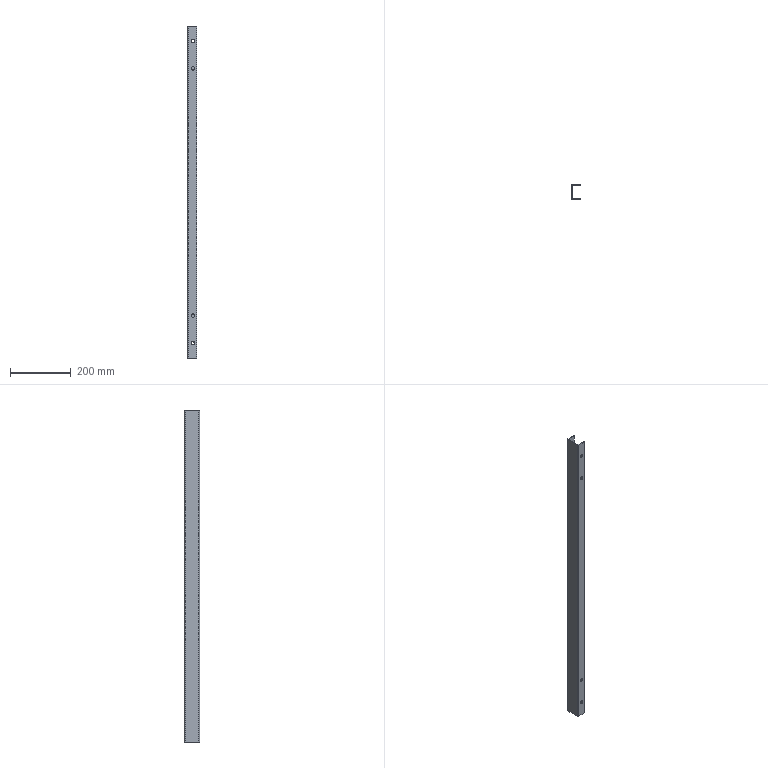Part | SolidWorks | features Cut 1, FlatPattern 1, ICE 1, SMBaseFlange 1, SheetMetal 1 | 1 solid | 55 faces | box 30 x 50 x 1095 mm | volume 331528 mm3 | plane 28 | cylinder 27 | commonest cylinder face diameters 10 x15 11 x8 0.4 x2 6.4 x2